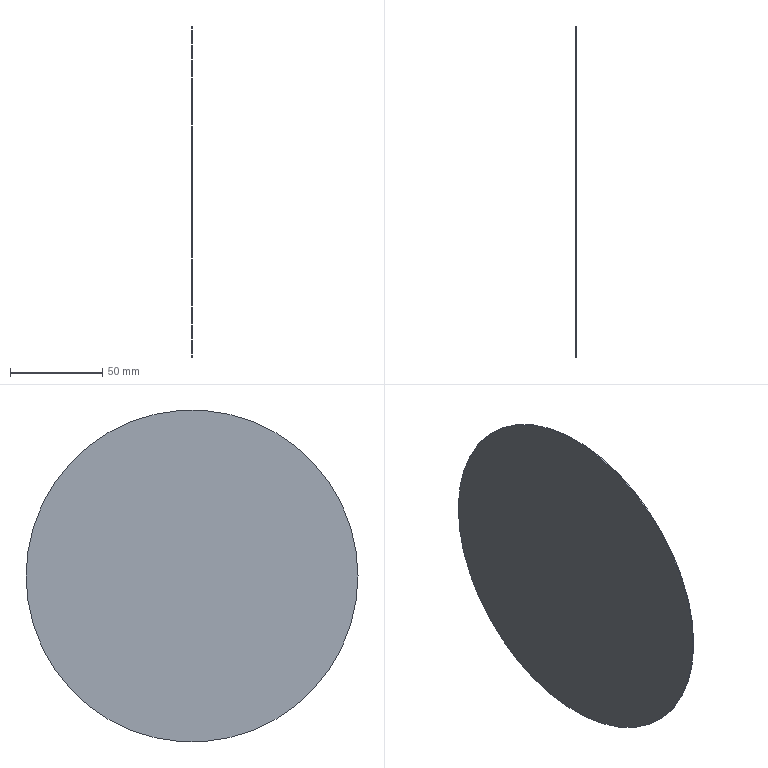Part | STEP file | Input 105 | 1 solid | 4 faces | box 0.5 x 180 x 180 mm | volume 12723 mm3 | cylinder 2 | plane 2 | commonest cylinder face diameters 180 x2
STEP:
#1=CARTESIAN_POINT('',(0.,0.,0.));
#2=DIRECTION('',(0.,0.,1.));
#3=DIRECTION('',(1.,0.,0.));
#4=AXIS2_PLACEMENT_3D('',#1,#2,#3);
#5=CARTESIAN_POINT('',(3719.,620.,-78.349));
#6=VERTEX_POINT('',#5);
#7=CARTESIAN_POINT('',(3719.,710.,77.536));
#8=VERTEX_POINT('',#7);
#9=CARTESIAN_POINT('',(3719.,665.,-0.4063));
#10=DIRECTION('',(-1.,0.,0.));
#11=DIRECTION('',(0.,-0.5,-0.866));
#12=AXIS2_PLACEMENT_3D('',#9,#10,#11);
#13=CIRCLE('',#12,90.);
#14=CARTESIAN_POINT('',(3719.,665.,-0.4063));
#15=DIRECTION('',(-1.,0.,0.));
#16=DIRECTION('',(0.,-0.5,-0.866));
#17=AXIS2_PLACEMENT_3D('',#14,#15,#16);
#18=CYLINDRICAL_SURFACE('',#17,90.);
#19=CARTESIAN_POINT('',(0.,0.));
#20=DIRECTION('',(1.,0.));
#21=VECTOR('',#20,1.);
#22=LINE('',#19,#21);
#23=(GEOMETRIC_REPRESENTATION_CONTEXT(2)PARAMETRIC_REPRESENTATION_CONTEXT()REPRESENTATION_CONTEXT('',''));
#24=DEFINITIONAL_REPRESENTATION('',(#22),#23);
#25=PCURVE('',#18,#24);
#26=CARTESIAN_POINT('',(3719.,665.,-0.4063));
#27=DIRECTION('',(1.,0.,0.));
#28=DIRECTION('',(0.,0.5,0.866));
#29=AXIS2_PLACEMENT_3D('',#26,#27,#28);
#30=PLANE('',#29);
#31=CARTESIAN_POINT('',(-90.,0.));
#32=CARTESIAN_POINT('',(-90.,155.885));
#33=CARTESIAN_POINT('',(45.,77.942));
#34=CARTESIAN_POINT('',(180.,0.));
#35=CARTESIAN_POINT('',(45.,-77.942));
#36=CARTESIAN_POINT('',(-90.,-155.885));
#37=CARTESIAN_POINT('',(-90.,0.));
#38=(BOUNDED_CURVE()B_SPLINE_CURVE(2,(#31,#32,#33,#34,#35,#36,#37),.UNSPECIFIED.,.T.,.F.)B_SPLINE_CURVE_WITH_KNOTS((1,2,2,2,2,1),(-2.094,0.,2.094,4.189,6.283,8.378),.UNSPECIFIED.)CURVE()GEOMETRIC_REPRESENTATION_ITEM()RATIONAL_B_SPLINE_CURVE((1.,0.5,1.,0.5,1.,0.5,1.))REPRESENTATION_ITEM(''));
#39=(GEOMETRIC_REPRESENTATION_CONTEXT(2)PARAMETRIC_REPRESENTATION_CONTEXT()REPRESENTATION_CONTEXT('',''));
#40=DEFINITIONAL_REPRESENTATION('',(#38),#39);
#41=PCURVE('',#30,#40);
#42=SURFACE_CURVE('',#13,(#25,#41),.PCURVE_S1.);
#43=EDGE_CURVE('',#6,#8,#42,.T.);
#44=ORIENTED_EDGE('',*,*,#43,.T.);
#45=CARTESIAN_POINT('',(3718.5,710.,77.536));
#46=VERTEX_POINT('',#45);
#47=CARTESIAN_POINT('',(3719.,710.,77.536));
#48=DIRECTION('',(-1.,0.,0.));
#49=VECTOR('',#48,1.);
#50=LINE('',#47,#49);
#51=CARTESIAN_POINT('',(3.142,0.));
#52=DIRECTION('',(0.,1.));
#53=VECTOR('',#52,1.);
#54=LINE('',#51,#53);
#55=(GEOMETRIC_REPRESENTATION_CONTEXT(2)PARAMETRIC_REPRESENTATION_CONTEXT()REPRESENTATION_CONTEXT('',''));
#56=DEFINITIONAL_REPRESENTATION('',(#54),#55);
#57=PCURVE('',#18,#56);
#58=CARTESIAN_POINT('',(3719.,665.,-0.4063));
#59=DIRECTION('',(-1.,0.,0.));
#60=DIRECTION('',(0.,-0.5,-0.866));
#61=AXIS2_PLACEMENT_3D('',#58,#59,#60);
#62=CYLINDRICAL_SURFACE('',#61,90.);
#63=CARTESIAN_POINT('',(3.142,0.));
#64=DIRECTION('',(0.,1.));
#65=VECTOR('',#64,1.);
#66=LINE('',#63,#65);
#67=(GEOMETRIC_REPRESENTATION_CONTEXT(2)PARAMETRIC_REPRESENTATION_CONTEXT()REPRESENTATION_CONTEXT('',''));
#68=DEFINITIONAL_REPRESENTATION('',(#66),#67);
#69=PCURVE('',#62,#68);
#70=SURFACE_CURVE('',#50,(#57,#69),.PCURVE_S1.);
#71=EDGE_CURVE('',#8,#46,#70,.T.);
#72=ORIENTED_EDGE('',*,*,#71,.T.);
#73=CARTESIAN_POINT('',(3718.5,620.,-78.349));
#74=VERTEX_POINT('',#73);
#75=CARTESIAN_POINT('',(3718.5,665.,-0.4063));
#76=DIRECTION('',(1.,0.,0.));
#77=DIRECTION('',(0.,0.5,0.866));
#78=AXIS2_PLACEMENT_3D('',#75,#76,#77);
#79=CIRCLE('',#78,90.);
#80=CARTESIAN_POINT('',(3.142,0.5));
#81=DIRECTION('',(-1.,0.));
#82=VECTOR('',#81,1.);
#83=LINE('',#80,#82);
#84=(GEOMETRIC_REPRESENTATION_CONTEXT(2)PARAMETRIC_REPRESENTATION_CONTEXT()REPRESENTATION_CONTEXT('',''));
#85=DEFINITIONAL_REPRESENTATION('',(#83),#84);
#86=PCURVE('',#18,#85);
#87=CARTESIAN_POINT('',(3718.5,665.,-0.4063));
#88=DIRECTION('',(-1.,0.,0.));
#89=DIRECTION('',(0.,-0.5,-0.866));
#90=AXIS2_PLACEMENT_3D('',#87,#88,#89);
#91=PLANE('',#90);
#92=CARTESIAN_POINT('',(-90.,0.));
#93=CARTESIAN_POINT('',(-90.,155.885));
#94=CARTESIAN_POINT('',(45.,77.942));
#95=CARTESIAN_POINT('',(180.,0.));
#96=CARTESIAN_POINT('',(45.,-77.942));
#97=CARTESIAN_POINT('',(-90.,-155.885));
#98=CARTESIAN_POINT('',(-90.,0.));
#99=(BOUNDED_CURVE()B_SPLINE_CURVE(2,(#92,#93,#94,#95,#96,#97,#98),.UNSPECIFIED.,.T.,.F.)B_SPLINE_CURVE_WITH_KNOTS((1,2,2,2,2,1),(-2.094,0.,2.094,4.189,6.283,8.378),.UNSPECIFIED.)CURVE()GEOMETRIC_REPRESENTATION_ITEM()RATIONAL_B_SPLINE_CURVE((1.,0.5,1.,0.5,1.,0.5,1.))REPRESENTATION_ITEM(''));
#100=(GEOMETRIC_REPRESENTATION_CONTEXT(2)PARAMETRIC_REPRESENTATION_CONTEXT()REPRESENTATION_CONTEXT('',''));
#101=DEFINITIONAL_REPRESENTATION('',(#99),#100);
#102=PCURVE('',#91,#101);
#103=SURFACE_CURVE('',#79,(#86,#102),.PCURVE_S1.);
#104=EDGE_CURVE('',#46,#74,#103,.T.);
#105=ORIENTED_EDGE('',*,*,#104,.T.);
#106=CARTESIAN_POINT('',(3719.,620.,-78.349));
#107=DIRECTION('',(-1.,0.,0.));
#108=VECTOR('',#107,1.);
#109=LINE('',#106,#108);
#110=CARTESIAN_POINT('',(0.,0.));
#111=DIRECTION('',(0.,1.));
#112=VECTOR('',#111,1.);
#113=LINE('',#110,#112);
#114=(GEOMETRIC_REPRESENTATION_CONTEXT(2)PARAMETRIC_REPRESENTATION_CONTEXT()REPRESENTATION_CONTEXT('',''));
#115=DEFINITIONAL_REPRESENTATION('',(#113),#114);
#116=PCURVE('',#18,#115);
#117=CARTESIAN_POINT('',(6.283,0.));
#118=DIRECTION('',(0.,1.));
#119=VECTOR('',#118,1.);
#120=LINE('',#117,#119);
#121=(GEOMETRIC_REPRESENTATION_CONTEXT(2)PARAMETRIC_REPRESENTATION_CONTEXT()REPRESENTATION_CONTEXT('',''));
#122=DEFINITIONAL_REPRESENTATION('',(#120),#121);
#123=PCURVE('',#62,#122);
#124=SURFACE_CURVE('',#109,(#116,#123),.PCURVE_S1.);
#125=EDGE_CURVE('',#6,#74,#124,.T.);
#126=ORIENTED_EDGE('',*,*,#125,.F.);
#127=EDGE_LOOP('',(#44,#72,#105,#126));
#128=FACE_BOUND('',#127,.T.);
#129=ADVANCED_FACE('',(#128),#18,.T.);
#130=CARTESIAN_POINT('',(3718.5,665.,-0.4063));
#131=DIRECTION('',(1.,0.,0.));
#132=DIRECTION('',(0.,0.5,0.866));
#133=AXIS2_PLACEMENT_3D('',#130,#131,#132);
#134=CIRCLE('',#133,90.);
#135=CARTESIAN_POINT('',(-90.,0.));
#136=CARTESIAN_POINT('',(-90.,155.885));
#137=CARTESIAN_POINT('',(45.,77.942));
#138=CARTESIAN_POINT('',(180.,0.));
#139=CARTESIAN_POINT('',(45.,-77.942));
#140=CARTESIAN_POINT('',(-90.,-155.885));
#141=CARTESIAN_POINT('',(-90.,0.));
#142=(BOUNDED_CURVE()B_SPLINE_CURVE(2,(#135,#136,#137,#138,#139,#140,#141),.UNSPECIFIED.,.T.,.F.)B_SPLINE_CURVE_WITH_KNOTS((1,2,2,2,2,1),(-2.094,0.,2.094,4.189,6.283,8.378),.UNSPECIFIED.)CURVE()GEOMETRIC_REPRESENTATION_ITEM()RATIONAL_B_SPLINE_CURVE((1.,0.5,1.,0.5,1.,0.5,1.))REPRESENTATION_ITEM(''));
#143=(GEOMETRIC_REPRESENTATION_CONTEXT(2)PARAMETRIC_REPRESENTATION_CONTEXT()REPRESENTATION_CONTEXT('',''));
#144=DEFINITIONAL_REPRESENTATION('',(#142),#143);
#145=PCURVE('',#91,#144);
#146=CARTESIAN_POINT('',(9.425,0.5));
#147=DIRECTION('',(-1.,0.));
#148=VECTOR('',#147,1.);
#149=LINE('',#146,#148);
#150=(GEOMETRIC_REPRESENTATION_CONTEXT(2)PARAMETRIC_REPRESENTATION_CONTEXT()REPRESENTATION_CONTEXT('',''));
#151=DEFINITIONAL_REPRESENTATION('',(#149),#150);
#152=PCURVE('',#62,#151);
#153=SURFACE_CURVE('',#134,(#145,#152),.PCURVE_S1.);
#154=EDGE_CURVE('',#74,#46,#153,.T.);
#155=ORIENTED_EDGE('',*,*,#154,.F.);
#156=ORIENTED_EDGE('',*,*,#104,.F.);
#157=EDGE_LOOP('',(#155,#156));
#158=FACE_BOUND('',#157,.T.);
#159=ADVANCED_FACE('',(#158),#91,.T.);
#160=ORIENTED_EDGE('',*,*,#43,.F.);
#161=CARTESIAN_POINT('',(3719.,665.,-0.4063));
#162=DIRECTION('',(-1.,0.,0.));
#163=DIRECTION('',(0.,-0.5,-0.866));
#164=AXIS2_PLACEMENT_3D('',#161,#162,#163);
#165=CIRCLE('',#164,90.);
#166=CARTESIAN_POINT('',(-90.,0.));
#167=CARTESIAN_POINT('',(-90.,155.885));
#168=CARTESIAN_POINT('',(45.,77.942));
#169=CARTESIAN_POINT('',(180.,0.));
#170=CARTESIAN_POINT('',(45.,-77.942));
#171=CARTESIAN_POINT('',(-90.,-155.885));
#172=CARTESIAN_POINT('',(-90.,0.));
#173=(BOUNDED_CURVE()B_SPLINE_CURVE(2,(#166,#167,#168,#169,#170,#171,#172),.UNSPECIFIED.,.T.,.F.)B_SPLINE_CURVE_WITH_KNOTS((1,2,2,2,2,1),(-2.094,0.,2.094,4.189,6.283,8.378),.UNSPECIFIED.)CURVE()GEOMETRIC_REPRESENTATION_ITEM()RATIONAL_B_SPLINE_CURVE((1.,0.5,1.,0.5,1.,0.5,1.))REPRESENTATION_ITEM(''));
#174=(GEOMETRIC_REPRESENTATION_CONTEXT(2)PARAMETRIC_REPRESENTATION_CONTEXT()REPRESENTATION_CONTEXT('',''));
#175=DEFINITIONAL_REPRESENTATION('',(#173),#174);
#176=PCURVE('',#30,#175);
#177=CARTESIAN_POINT('',(0.,0.));
#178=DIRECTION('',(1.,0.));
#179=VECTOR('',#178,1.);
#180=LINE('',#177,#179);
#181=(GEOMETRIC_REPRESENTATION_CONTEXT(2)PARAMETRIC_REPRESENTATION_CONTEXT()REPRESENTATION_CONTEXT('',''));
#182=DEFINITIONAL_REPRESENTATION('',(#180),#181);
#183=PCURVE('',#62,#182);
#184=SURFACE_CURVE('',#165,(#176,#183),.PCURVE_S1.);
#185=EDGE_CURVE('',#8,#6,#184,.T.);
#186=ORIENTED_EDGE('',*,*,#185,.F.);
#187=EDGE_LOOP('',(#160,#186));
#188=FACE_BOUND('',#187,.T.);
#189=ADVANCED_FACE('',(#188),#30,.T.);
#190=ORIENTED_EDGE('',*,*,#71,.F.);
#191=ORIENTED_EDGE('',*,*,#185,.T.);
#192=ORIENTED_EDGE('',*,*,#125,.T.);
#193=ORIENTED_EDGE('',*,*,#154,.T.);
#194=EDGE_LOOP('',(#190,#191,#192,#193));
#195=FACE_BOUND('',#194,.T.);
#196=ADVANCED_FACE('',(#195),#62,.T.);
#197=CLOSED_SHELL('',(#129,#159,#189,#196));
#198=MANIFOLD_SOLID_BREP('',#197);
#199=(LENGTH_UNIT()NAMED_UNIT(*)SI_UNIT(.MILLI.,.METRE.));
#200=UNCERTAINTY_MEASURE_WITH_UNIT(LENGTH_MEASURE(0.0000001),#199,'','');
#201=(NAMED_UNIT(*)PLANE_ANGLE_UNIT()SI_UNIT($,.RADIAN.));
#202=(NAMED_UNIT(*)SI_UNIT($,.STERADIAN.)SOLID_ANGLE_UNIT());
#203=(GEOMETRIC_REPRESENTATION_CONTEXT(3)GLOBAL_UNCERTAINTY_ASSIGNED_CONTEXT((#200))GLOBAL_UNIT_ASSIGNED_CONTEXT((#199,#201,#202))REPRESENTATION_CONTEXT('',''));
#204=ADVANCED_BREP_SHAPE_REPRESENTATION('',(#4,#198),#203);